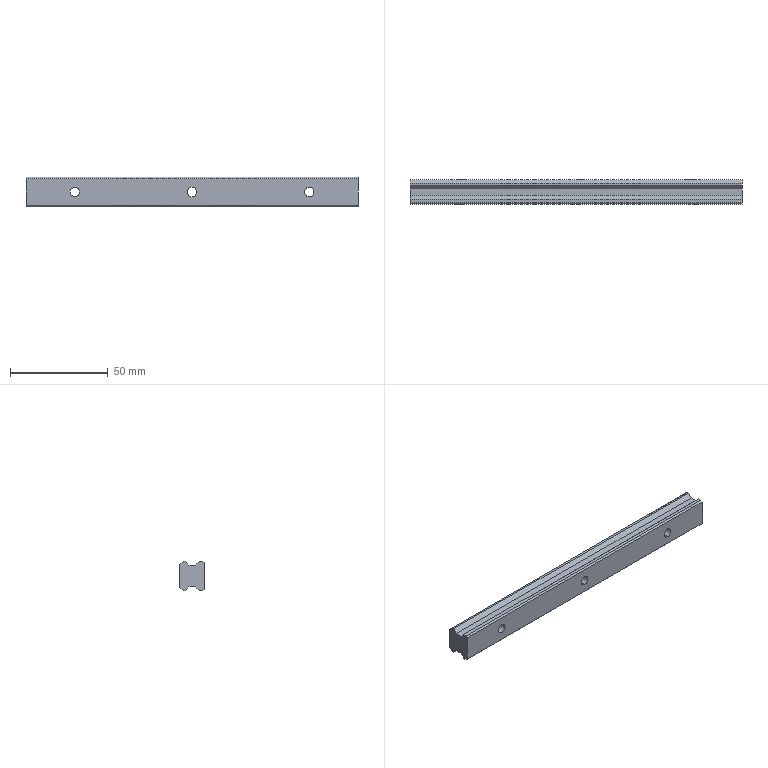Part | STEP file | LSD15RLX170-S25-N-D | 1 solid | 33 faces | box 170 x 12.5 x 15 mm | volume 26475 mm3 | plane 21 | cylinder 12 | commonest cylinder face diameters 4.8 x6 8 x6